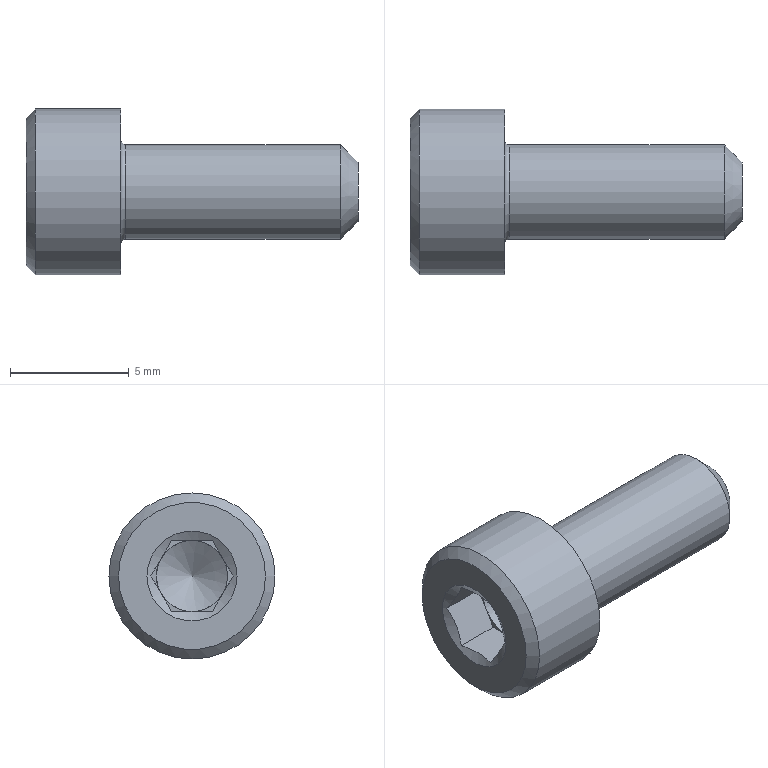Part | STEP file | Винт М4-6gx10 ГОСТ 11738-84 | 1 solid | 23 faces | box 14 x 7 x 7 mm | volume 252.721 mm3 | plane 15 | cone 4 | cylinder 3 | torus 1 | commonest cylinder face diameters 3 x1 4 x1 7 x1
STEP:
#1=CARTESIAN_POINT('',(-4.,3.1,0.));
#2=VERTEX_POINT('',#1);
#3=CARTESIAN_POINT('',(-4.,0.,0.));
#4=DIRECTION('',(1.,0.,0.));
#5=DIRECTION('',(0.,1.,0.));
#6=AXIS2_PLACEMENT_3D('',#3,#4,#5);
#7=CIRCLE('',#6,3.1);
#8=EDGE_CURVE('',#2,#2,#7,.T.);
#9=ORIENTED_EDGE('',*,*,#8,.F.);
#10=EDGE_LOOP('',(#9));
#11=FACE_BOUND('',#10,.T.);
#12=CARTESIAN_POINT('',(-4.,1.9,0.));
#13=VERTEX_POINT('',#12);
#14=CARTESIAN_POINT('',(-4.,0.,0.));
#15=DIRECTION('',(1.,0.,0.));
#16=DIRECTION('',(0.,1.,0.));
#17=AXIS2_PLACEMENT_3D('',#14,#15,#16);
#18=CIRCLE('',#17,1.9);
#19=EDGE_CURVE('',#13,#13,#18,.T.);
#20=ORIENTED_EDGE('',*,*,#19,.T.);
#21=EDGE_LOOP('',(#20));
#22=FACE_BOUND('',#21,.T.);
#23=CARTESIAN_POINT('',(-4.,0.,0.));
#24=DIRECTION('',(-1.,0.,0.));
#25=DIRECTION('',(0.,1.,0.));
#26=AXIS2_PLACEMENT_3D('',#23,#24,#25);
#27=PLANE('',#26);
#28=ADVANCED_FACE('',(#11,#22),#27,.T.);
#29=CARTESIAN_POINT('',(-3.903,0.866,-1.5));
#30=VERTEX_POINT('',#29);
#31=CARTESIAN_POINT('',(-3.903,-0.866,-1.5));
#32=VERTEX_POINT('',#31);
#33=CARTESIAN_POINT('',(-3.903,0.866,-1.5));
#34=CARTESIAN_POINT('',(-3.9,0.8561,-1.5));
#35=CARTESIAN_POINT('',(-3.89,0.8205,-1.5));
#36=CARTESIAN_POINT('',(-3.88,0.7841,-1.5));
#37=CARTESIAN_POINT('',(-3.862,0.7149,-1.5));
#38=CARTESIAN_POINT('',(-3.851,0.6675,-1.5));
#39=CARTESIAN_POINT('',(-3.83,0.5736,-1.5));
#40=CARTESIAN_POINT('',(-3.816,0.5059,-1.5));
#41=CARTESIAN_POINT('',(-3.8,0.4061,-1.5));
#42=CARTESIAN_POINT('',(-3.789,0.3305,-1.5));
#43=CARTESIAN_POINT('',(-3.781,0.2553,-1.5));
#44=CARTESIAN_POINT('',(-3.776,0.1888,-1.5));
#45=CARTESIAN_POINT('',(-3.773,0.1381,-1.5));
#46=CARTESIAN_POINT('',(-3.771,0.09396,-1.5));
#47=CARTESIAN_POINT('',(-3.77,0.0601,-1.5));
#48=CARTESIAN_POINT('',(-3.769,0.0279,-1.5));
#49=CARTESIAN_POINT('',(-3.769,-0.005342,-1.5));
#50=CARTESIAN_POINT('',(-3.769,-0.03809,-1.5));
#51=CARTESIAN_POINT('',(-3.77,-0.07339,-1.5));
#52=CARTESIAN_POINT('',(-3.771,-0.1059,-1.5));
#53=CARTESIAN_POINT('',(-3.773,-0.1382,-1.5));
#54=CARTESIAN_POINT('',(-3.775,-0.1786,-1.5));
#55=CARTESIAN_POINT('',(-3.779,-0.2268,-1.5));
#56=CARTESIAN_POINT('',(-3.783,-0.2747,-1.5));
#57=CARTESIAN_POINT('',(-3.788,-0.3143,-1.5));
#58=CARTESIAN_POINT('',(-3.792,-0.346,-1.5));
#59=CARTESIAN_POINT('',(-3.796,-0.3774,-1.5));
#60=CARTESIAN_POINT('',(-3.802,-0.4165,-1.5));
#61=CARTESIAN_POINT('',(-3.809,-0.463,-1.5));
#62=CARTESIAN_POINT('',(-3.817,-0.5065,-1.5));
#63=CARTESIAN_POINT('',(-3.823,-0.5371,-1.5));
#64=CARTESIAN_POINT('',(-3.829,-0.5675,-1.5));
#65=CARTESIAN_POINT('',(-3.836,-0.6003,-1.5));
#66=CARTESIAN_POINT('',(-3.846,-0.6453,-1.5));
#67=CARTESIAN_POINT('',(-3.856,-0.69,-1.5));
#68=CARTESIAN_POINT('',(-3.865,-0.7249,-1.5));
#69=CARTESIAN_POINT('',(-3.872,-0.7544,-1.5));
#70=CARTESIAN_POINT('',(-3.88,-0.7837,-1.5));
#71=CARTESIAN_POINT('',(-3.891,-0.8224,-1.5));
#72=CARTESIAN_POINT('',(-3.899,-0.8515,-1.5));
#73=CARTESIAN_POINT('',(-3.903,-0.866,-1.5));
#74=B_SPLINE_CURVE_WITH_KNOTS('',3,(#33,#34,#35,#36,#37,#38,#39,#40,#41,#42,#43,#44,#45,#46,#47,#48,#49,#50,#51,#52,#53,#54,#55,#56,#57,#58,#59,#60,#61,#62,#63,#64,#65,#66,#67,#68,#69,#70,#71,#72,#73),.UNSPECIFIED.,.F.,.F.,(4,1,1,1,1,1,1,1,1,1,1,1,1,1,1,1,1,1,1,1,1,1,1,1,1,1,1,1,1,1,1,1,1,1,1,1,1,1,4),(0.,0.01755,0.06316,0.06435,0.1397,0.1462,0.2284,0.2575,0.3188,0.3585,0.3865,0.4328,0.4451,0.4618,0.4905,0.5,0.5185,0.5464,0.5602,0.574,0.6016,0.6291,0.6565,0.6838,0.6972,0.7109,0.7379,0.7646,0.7912,0.8132,0.8177,0.8441,0.8703,0.8963,0.9224,0.9317,0.9483,0.9741,1.),.UNSPECIFIED.);
#75=EDGE_CURVE('',#30,#32,#74,.T.);
#76=ORIENTED_EDGE('',*,*,#75,.T.);
#77=CARTESIAN_POINT('',(-2.,-0.866,-1.5));
#78=VERTEX_POINT('',#77);
#79=CARTESIAN_POINT('',(-2.,-0.866,-1.5));
#80=DIRECTION('',(-1.,0.,0.));
#81=VECTOR('',#80,1.);
#82=LINE('',#79,#81);
#83=EDGE_CURVE('',#78,#32,#82,.T.);
#84=ORIENTED_EDGE('',*,*,#83,.F.);
#85=CARTESIAN_POINT('',(-2.,0.,-1.5));
#86=VERTEX_POINT('',#85);
#87=CARTESIAN_POINT('',(-2.,0.,-1.5));
#88=DIRECTION('',(0.,-1.,0.));
#89=VECTOR('',#88,1.);
#90=LINE('',#87,#89);
#91=EDGE_CURVE('',#86,#78,#90,.T.);
#92=ORIENTED_EDGE('',*,*,#91,.F.);
#93=CARTESIAN_POINT('',(-2.,0.866,-1.5));
#94=VERTEX_POINT('',#93);
#95=CARTESIAN_POINT('',(-2.,0.866,-1.5));
#96=DIRECTION('',(0.,-1.,0.));
#97=VECTOR('',#96,1.);
#98=LINE('',#95,#97);
#99=EDGE_CURVE('',#94,#86,#98,.T.);
#100=ORIENTED_EDGE('',*,*,#99,.F.);
#101=CARTESIAN_POINT('',(-2.,0.866,-1.5));
#102=DIRECTION('',(-1.,0.,0.));
#103=VECTOR('',#102,1.);
#104=LINE('',#101,#103);
#105=EDGE_CURVE('',#94,#30,#104,.T.);
#106=ORIENTED_EDGE('',*,*,#105,.T.);
#107=EDGE_LOOP('',(#76,#84,#92,#100,#106));
#108=FACE_BOUND('',#107,.T.);
#109=CARTESIAN_POINT('',(-2.,0.866,-1.5));
#110=DIRECTION('',(0.,0.,-1.));
#111=DIRECTION('',(0.,-1.,0.));
#112=AXIS2_PLACEMENT_3D('',#109,#110,#111);
#113=PLANE('',#112);
#114=ADVANCED_FACE('',(#108),#113,.F.);
#115=CARTESIAN_POINT('',(-3.903,-1.732,0.));
#116=VERTEX_POINT('',#115);
#117=CARTESIAN_POINT('',(-3.903,-0.866,-1.5));
#118=CARTESIAN_POINT('',(-3.893,-0.8838,-1.469));
#119=CARTESIAN_POINT('',(-3.871,-0.9233,-1.401));
#120=CARTESIAN_POINT('',(-3.839,-0.9883,-1.288));
#121=CARTESIAN_POINT('',(-3.81,-1.062,-1.161));
#122=CARTESIAN_POINT('',(-3.789,-1.133,-1.037));
#123=CARTESIAN_POINT('',(-3.777,-1.193,-0.9336));
#124=CARTESIAN_POINT('',(-3.772,-1.235,-0.8611));
#125=CARTESIAN_POINT('',(-3.77,-1.265,-0.8083));
#126=CARTESIAN_POINT('',(-3.769,-1.285,-0.7742));
#127=CARTESIAN_POINT('',(-3.769,-1.302,-0.7454));
#128=CARTESIAN_POINT('',(-3.769,-1.318,-0.717));
#129=CARTESIAN_POINT('',(-3.77,-1.34,-0.6794));
#130=CARTESIAN_POINT('',(-3.772,-1.364,-0.6373));
#131=CARTESIAN_POINT('',(-3.775,-1.388,-0.5954));
#132=CARTESIAN_POINT('',(-3.779,-1.412,-0.5536));
#133=CARTESIAN_POINT('',(-3.783,-1.436,-0.5121));
#134=CARTESIAN_POINT('',(-3.789,-1.46,-0.4709));
#135=CARTESIAN_POINT('',(-3.795,-1.484,-0.4299));
#136=CARTESIAN_POINT('',(-3.802,-1.507,-0.3893));
#137=CARTESIAN_POINT('',(-3.809,-1.531,-0.349));
#138=CARTESIAN_POINT('',(-3.817,-1.554,-0.3091));
#139=CARTESIAN_POINT('',(-3.826,-1.576,-0.2695));
#140=CARTESIAN_POINT('',(-3.836,-1.599,-0.2301));
#141=CARTESIAN_POINT('',(-3.846,-1.622,-0.1912));
#142=CARTESIAN_POINT('',(-3.856,-1.644,-0.1525));
#143=CARTESIAN_POINT('',(-3.867,-1.666,-0.114));
#144=CARTESIAN_POINT('',(-3.879,-1.688,-0.07582));
#145=CARTESIAN_POINT('',(-3.891,-1.71,-0.03781));
#146=CARTESIAN_POINT('',(-3.899,-1.725,-0.01258));
#147=CARTESIAN_POINT('',(-3.903,-1.732,0.));
#148=B_SPLINE_CURVE_WITH_KNOTS('',3,(#117,#118,#119,#120,#121,#122,#123,#124,#125,#126,#127,#128,#129,#130,#131,#132,#133,#134,#135,#136,#137,#138,#139,#140,#141,#142,#143,#144,#145,#146,#147),.UNSPECIFIED.,.F.,.F.,(4,1,1,1,1,1,1,1,1,1,1,1,1,1,1,1,1,1,1,1,1,1,1,1,1,1,1,1,4),(0.,0.06316,0.1397,0.2284,0.3188,0.3865,0.4328,0.4618,0.4905,0.5,0.5185,0.5464,0.574,0.6016,0.6291,0.6565,0.6838,0.7109,0.7379,0.7646,0.7912,0.8177,0.8441,0.8703,0.8963,0.9224,0.9483,0.9741,1.),.UNSPECIFIED.);
#149=EDGE_CURVE('',#32,#116,#148,.T.);
#150=ORIENTED_EDGE('',*,*,#149,.T.);
#151=CARTESIAN_POINT('',(-2.,-1.732,0.));
#152=VERTEX_POINT('',#151);
#153=CARTESIAN_POINT('',(-2.,-1.732,0.));
#154=DIRECTION('',(-1.,0.,0.));
#155=VECTOR('',#154,1.);
#156=LINE('',#153,#155);
#157=EDGE_CURVE('',#152,#116,#156,.T.);
#158=ORIENTED_EDGE('',*,*,#157,.F.);
#159=CARTESIAN_POINT('',(-2.,-1.299,-0.75));
#160=VERTEX_POINT('',#159);
#161=CARTESIAN_POINT('',(-2.,-1.299,-0.75));
#162=DIRECTION('',(0.,-0.5,0.866));
#163=VECTOR('',#162,1.);
#164=LINE('',#161,#163);
#165=EDGE_CURVE('',#160,#152,#164,.T.);
#166=ORIENTED_EDGE('',*,*,#165,.F.);
#167=CARTESIAN_POINT('',(-2.,-0.866,-1.5));
#168=DIRECTION('',(0.,-0.5,0.866));
#169=VECTOR('',#168,1.);
#170=LINE('',#167,#169);
#171=EDGE_CURVE('',#78,#160,#170,.T.);
#172=ORIENTED_EDGE('',*,*,#171,.F.);
#173=ORIENTED_EDGE('',*,*,#83,.T.);
#174=EDGE_LOOP('',(#150,#158,#166,#172,#173));
#175=FACE_BOUND('',#174,.T.);
#176=CARTESIAN_POINT('',(-2.,-0.866,-1.5));
#177=DIRECTION('',(0.,-0.866,-0.5));
#178=DIRECTION('',(0.,-0.5,0.866));
#179=AXIS2_PLACEMENT_3D('',#176,#177,#178);
#180=PLANE('',#179);
#181=ADVANCED_FACE('',(#175),#180,.F.);
#182=CARTESIAN_POINT('',(-3.903,-0.866,1.5));
#183=VERTEX_POINT('',#182);
#184=CARTESIAN_POINT('',(-3.903,-1.732,0.));
#185=CARTESIAN_POINT('',(-3.893,-1.714,0.0308));
#186=CARTESIAN_POINT('',(-3.871,-1.675,0.09916));
#187=CARTESIAN_POINT('',(-3.839,-1.61,0.2118));
#188=CARTESIAN_POINT('',(-3.81,-1.536,0.3391));
#189=CARTESIAN_POINT('',(-3.789,-1.465,0.4631));
#190=CARTESIAN_POINT('',(-3.777,-1.405,0.5664));
#191=CARTESIAN_POINT('',(-3.772,-1.363,0.6389));
#192=CARTESIAN_POINT('',(-3.77,-1.333,0.6917));
#193=CARTESIAN_POINT('',(-3.769,-1.313,0.7258));
#194=CARTESIAN_POINT('',(-3.769,-1.296,0.7546));
#195=CARTESIAN_POINT('',(-3.769,-1.28,0.783));
#196=CARTESIAN_POINT('',(-3.77,-1.258,0.8206));
#197=CARTESIAN_POINT('',(-3.772,-1.234,0.8627));
#198=CARTESIAN_POINT('',(-3.775,-1.21,0.9046));
#199=CARTESIAN_POINT('',(-3.779,-1.186,0.9464));
#200=CARTESIAN_POINT('',(-3.783,-1.162,0.9879));
#201=CARTESIAN_POINT('',(-3.789,-1.138,1.029));
#202=CARTESIAN_POINT('',(-3.795,-1.114,1.07));
#203=CARTESIAN_POINT('',(-3.802,-1.091,1.111));
#204=CARTESIAN_POINT('',(-3.809,-1.068,1.151));
#205=CARTESIAN_POINT('',(-3.817,-1.044,1.191));
#206=CARTESIAN_POINT('',(-3.826,-1.022,1.231));
#207=CARTESIAN_POINT('',(-3.836,-0.9989,1.27));
#208=CARTESIAN_POINT('',(-3.846,-0.9764,1.309));
#209=CARTESIAN_POINT('',(-3.856,-0.954,1.348));
#210=CARTESIAN_POINT('',(-3.867,-0.9319,1.386));
#211=CARTESIAN_POINT('',(-3.879,-0.9098,1.424));
#212=CARTESIAN_POINT('',(-3.891,-0.8879,1.462));
#213=CARTESIAN_POINT('',(-3.899,-0.8733,1.487));
#214=CARTESIAN_POINT('',(-3.903,-0.866,1.5));
#215=B_SPLINE_CURVE_WITH_KNOTS('',3,(#184,#185,#186,#187,#188,#189,#190,#191,#192,#193,#194,#195,#196,#197,#198,#199,#200,#201,#202,#203,#204,#205,#206,#207,#208,#209,#210,#211,#212,#213,#214),.UNSPECIFIED.,.F.,.F.,(4,1,1,1,1,1,1,1,1,1,1,1,1,1,1,1,1,1,1,1,1,1,1,1,1,1,1,1,4),(0.,0.06316,0.1397,0.2284,0.3188,0.3865,0.4328,0.4618,0.4905,0.5,0.5185,0.5464,0.574,0.6016,0.6291,0.6565,0.6838,0.7109,0.7379,0.7646,0.7912,0.8177,0.8441,0.8703,0.8963,0.9224,0.9483,0.9741,1.),.UNSPECIFIED.);
#216=EDGE_CURVE('',#116,#183,#215,.T.);
#217=ORIENTED_EDGE('',*,*,#216,.T.);
#218=CARTESIAN_POINT('',(-2.,-0.866,1.5));
#219=VERTEX_POINT('',#218);
#220=CARTESIAN_POINT('',(-2.,-0.866,1.5));
#221=DIRECTION('',(-1.,0.,0.));
#222=VECTOR('',#221,1.);
#223=LINE('',#220,#222);
#224=EDGE_CURVE('',#219,#183,#223,.T.);
#225=ORIENTED_EDGE('',*,*,#224,.F.);
#226=CARTESIAN_POINT('',(-2.,-1.299,0.75));
#227=VERTEX_POINT('',#226);
#228=CARTESIAN_POINT('',(-2.,-1.299,0.75));
#229=DIRECTION('',(0.,0.5,0.866));
#230=VECTOR('',#229,1.);
#231=LINE('',#228,#230);
#232=EDGE_CURVE('',#227,#219,#231,.T.);
#233=ORIENTED_EDGE('',*,*,#232,.F.);
#234=CARTESIAN_POINT('',(-2.,-1.732,0.));
#235=DIRECTION('',(0.,0.5,0.866));
#236=VECTOR('',#235,1.);
#237=LINE('',#234,#236);
#238=EDGE_CURVE('',#152,#227,#237,.T.);
#239=ORIENTED_EDGE('',*,*,#238,.F.);
#240=ORIENTED_EDGE('',*,*,#157,.T.);
#241=EDGE_LOOP('',(#217,#225,#233,#239,#240));
#242=FACE_BOUND('',#241,.T.);
#243=CARTESIAN_POINT('',(-2.,-1.732,0.));
#244=DIRECTION('',(0.,-0.866,0.5));
#245=DIRECTION('',(0.,0.5,0.866));
#246=AXIS2_PLACEMENT_3D('',#243,#244,#245);
#247=PLANE('',#246);
#248=ADVANCED_FACE('',(#242),#247,.F.);
#249=CARTESIAN_POINT('',(-3.903,0.866,1.5));
#250=VERTEX_POINT('',#249);
#251=CARTESIAN_POINT('',(-3.903,-0.866,1.5));
#252=CARTESIAN_POINT('',(-3.9,-0.8561,1.5));
#253=CARTESIAN_POINT('',(-3.89,-0.8205,1.5));
#254=CARTESIAN_POINT('',(-3.88,-0.7841,1.5));
#255=CARTESIAN_POINT('',(-3.862,-0.7149,1.5));
#256=CARTESIAN_POINT('',(-3.851,-0.6675,1.5));
#257=CARTESIAN_POINT('',(-3.83,-0.5736,1.5));
#258=CARTESIAN_POINT('',(-3.816,-0.5059,1.5));
#259=CARTESIAN_POINT('',(-3.8,-0.4061,1.5));
#260=CARTESIAN_POINT('',(-3.789,-0.3305,1.5));
#261=CARTESIAN_POINT('',(-3.781,-0.2553,1.5));
#262=CARTESIAN_POINT('',(-3.776,-0.1888,1.5));
#263=CARTESIAN_POINT('',(-3.773,-0.1381,1.5));
#264=CARTESIAN_POINT('',(-3.771,-0.09396,1.5));
#265=CARTESIAN_POINT('',(-3.77,-0.0601,1.5));
#266=CARTESIAN_POINT('',(-3.769,-0.0279,1.5));
#267=CARTESIAN_POINT('',(-3.769,0.005342,1.5));
#268=CARTESIAN_POINT('',(-3.769,0.03809,1.5));
#269=CARTESIAN_POINT('',(-3.77,0.07339,1.5));
#270=CARTESIAN_POINT('',(-3.771,0.1059,1.5));
#271=CARTESIAN_POINT('',(-3.773,0.1382,1.5));
#272=CARTESIAN_POINT('',(-3.775,0.1786,1.5));
#273=CARTESIAN_POINT('',(-3.779,0.2268,1.5));
#274=CARTESIAN_POINT('',(-3.783,0.2747,1.5));
#275=CARTESIAN_POINT('',(-3.788,0.3143,1.5));
#276=CARTESIAN_POINT('',(-3.792,0.346,1.5));
#277=CARTESIAN_POINT('',(-3.796,0.3774,1.5));
#278=CARTESIAN_POINT('',(-3.802,0.4165,1.5));
#279=CARTESIAN_POINT('',(-3.809,0.463,1.5));
#280=CARTESIAN_POINT('',(-3.817,0.5065,1.5));
#281=CARTESIAN_POINT('',(-3.823,0.5371,1.5));
#282=CARTESIAN_POINT('',(-3.829,0.5675,1.5));
#283=CARTESIAN_POINT('',(-3.836,0.6003,1.5));
#284=CARTESIAN_POINT('',(-3.846,0.6453,1.5));
#285=CARTESIAN_POINT('',(-3.856,0.69,1.5));
#286=CARTESIAN_POINT('',(-3.865,0.7249,1.5));
#287=CARTESIAN_POINT('',(-3.872,0.7544,1.5));
#288=CARTESIAN_POINT('',(-3.88,0.7837,1.5));
#289=CARTESIAN_POINT('',(-3.891,0.8224,1.5));
#290=CARTESIAN_POINT('',(-3.899,0.8515,1.5));
#291=CARTESIAN_POINT('',(-3.903,0.866,1.5));
#292=B_SPLINE_CURVE_WITH_KNOTS('',3,(#251,#252,#253,#254,#255,#256,#257,#258,#259,#260,#261,#262,#263,#264,#265,#266,#267,#268,#269,#270,#271,#272,#273,#274,#275,#276,#277,#278,#279,#280,#281,#282,#283,#284,#285,#286,#287,#288,#289,#290,#291),.UNSPECIFIED.,.F.,.F.,(4,1,1,1,1,1,1,1,1,1,1,1,1,1,1,1,1,1,1,1,1,1,1,1,1,1,1,1,1,1,1,1,1,1,1,1,1,1,4),(0.,0.01755,0.06316,0.06435,0.1397,0.1462,0.2284,0.2575,0.3188,0.3585,0.3865,0.4328,0.4451,0.4618,0.4905,0.5,0.5185,0.5464,0.5602,0.574,0.6016,0.6291,0.6565,0.6838,0.6972,0.7109,0.7379,0.7646,0.7912,0.8132,0.8177,0.8441,0.8703,0.8963,0.9224,0.9317,0.9483,0.9741,1.),.UNSPECIFIED.);
#293=EDGE_CURVE('',#183,#250,#292,.T.);
#294=ORIENTED_EDGE('',*,*,#293,.T.);
#295=CARTESIAN_POINT('',(-2.,0.866,1.5));
#296=VERTEX_POINT('',#295);
#297=CARTESIAN_POINT('',(-2.,0.866,1.5));
#298=DIRECTION('',(-1.,0.,0.));
#299=VECTOR('',#298,1.);
#300=LINE('',#297,#299);
#301=EDGE_CURVE('',#296,#250,#300,.T.);
#302=ORIENTED_EDGE('',*,*,#301,.F.);
#303=CARTESIAN_POINT('',(-2.,0.,1.5));
#304=VERTEX_POINT('',#303);
#305=CARTESIAN_POINT('',(-2.,0.,1.5));
#306=DIRECTION('',(0.,1.,0.));
#307=VECTOR('',#306,1.);
#308=LINE('',#305,#307);
#309=EDGE_CURVE('',#304,#296,#308,.T.);
#310=ORIENTED_EDGE('',*,*,#309,.F.);
#311=CARTESIAN_POINT('',(-2.,-0.866,1.5));
#312=DIRECTION('',(0.,1.,0.));
#313=VECTOR('',#312,1.);
#314=LINE('',#311,#313);
#315=EDGE_CURVE('',#219,#304,#314,.T.);
#316=ORIENTED_EDGE('',*,*,#315,.F.);
#317=ORIENTED_EDGE('',*,*,#224,.T.);
#318=EDGE_LOOP('',(#294,#302,#310,#316,#317));
#319=FACE_BOUND('',#318,.T.);
#320=CARTESIAN_POINT('',(-2.,-0.866,1.5));
#321=DIRECTION('',(0.,0.,1.));
#322=DIRECTION('',(0.,1.,0.));
#323=AXIS2_PLACEMENT_3D('',#320,#321,#322);
#324=PLANE('',#323);
#325=ADVANCED_FACE('',(#319),#324,.F.);
#326=CARTESIAN_POINT('',(-3.903,1.732,0.000000001));
#327=VERTEX_POINT('',#326);
#328=CARTESIAN_POINT('',(-3.903,1.732,0.));
#329=CARTESIAN_POINT('',(-3.893,1.714,-0.0308));
#330=CARTESIAN_POINT('',(-3.871,1.675,-0.09916));
#331=CARTESIAN_POINT('',(-3.839,1.61,-0.2118));
#332=CARTESIAN_POINT('',(-3.81,1.536,-0.3391));
#333=CARTESIAN_POINT('',(-3.789,1.465,-0.4631));
#334=CARTESIAN_POINT('',(-3.777,1.405,-0.5664));
#335=CARTESIAN_POINT('',(-3.772,1.363,-0.6389));
#336=CARTESIAN_POINT('',(-3.77,1.333,-0.6917));
#337=CARTESIAN_POINT('',(-3.769,1.313,-0.7258));
#338=CARTESIAN_POINT('',(-3.769,1.296,-0.7546));
#339=CARTESIAN_POINT('',(-3.769,1.28,-0.783));
#340=CARTESIAN_POINT('',(-3.77,1.258,-0.8206));
#341=CARTESIAN_POINT('',(-3.772,1.234,-0.8627));
#342=CARTESIAN_POINT('',(-3.775,1.21,-0.9046));
#343=CARTESIAN_POINT('',(-3.779,1.186,-0.9464));
#344=CARTESIAN_POINT('',(-3.783,1.162,-0.9879));
#345=CARTESIAN_POINT('',(-3.789,1.138,-1.029));
#346=CARTESIAN_POINT('',(-3.795,1.114,-1.07));
#347=CARTESIAN_POINT('',(-3.802,1.091,-1.111));
#348=CARTESIAN_POINT('',(-3.809,1.068,-1.151));
#349=CARTESIAN_POINT('',(-3.817,1.044,-1.191));
#350=CARTESIAN_POINT('',(-3.826,1.022,-1.231));
#351=CARTESIAN_POINT('',(-3.836,0.9989,-1.27));
#352=CARTESIAN_POINT('',(-3.846,0.9764,-1.309));
#353=CARTESIAN_POINT('',(-3.856,0.954,-1.348));
#354=CARTESIAN_POINT('',(-3.867,0.9319,-1.386));
#355=CARTESIAN_POINT('',(-3.879,0.9098,-1.424));
#356=CARTESIAN_POINT('',(-3.891,0.8879,-1.462));
#357=CARTESIAN_POINT('',(-3.899,0.8733,-1.487));
#358=CARTESIAN_POINT('',(-3.903,0.866,-1.5));
#359=B_SPLINE_CURVE_WITH_KNOTS('',3,(#328,#329,#330,#331,#332,#333,#334,#335,#336,#337,#338,#339,#340,#341,#342,#343,#344,#345,#346,#347,#348,#349,#350,#351,#352,#353,#354,#355,#356,#357,#358),.UNSPECIFIED.,.F.,.F.,(4,1,1,1,1,1,1,1,1,1,1,1,1,1,1,1,1,1,1,1,1,1,1,1,1,1,1,1,4),(0.,0.06315,0.1397,0.2284,0.3188,0.3865,0.4327,0.4618,0.4905,0.5,0.5185,0.5464,0.574,0.6016,0.6291,0.6565,0.6838,0.7109,0.7379,0.7646,0.7912,0.8177,0.8441,0.8703,0.8963,0.9224,0.9483,0.9741,1.),.UNSPECIFIED.);
#360=EDGE_CURVE('',#327,#30,#359,.T.);
#361=ORIENTED_EDGE('',*,*,#360,.T.);
#362=ORIENTED_EDGE('',*,*,#105,.F.);
#363=CARTESIAN_POINT('',(-2.,1.299,-0.75));
#364=VERTEX_POINT('',#363);
#365=CARTESIAN_POINT('',(-2.,1.299,-0.75));
#366=DIRECTION('',(0.,-0.5,-0.866));
#367=VECTOR('',#366,1.);
#368=LINE('',#365,#367);
#369=EDGE_CURVE('',#364,#94,#368,.T.);
#370=ORIENTED_EDGE('',*,*,#369,.F.);
#371=CARTESIAN_POINT('',(-2.,1.732,0.));
#372=VERTEX_POINT('',#371);
#373=CARTESIAN_POINT('',(-2.,1.732,0.));
#374=DIRECTION('',(0.,-0.5,-0.866));
#375=VECTOR('',#374,1.);
#376=LINE('',#373,#375);
#377=EDGE_CURVE('',#372,#364,#376,.T.);
#378=ORIENTED_EDGE('',*,*,#377,.F.);
#379=CARTESIAN_POINT('',(-2.,1.732,0.));
#380=DIRECTION('',(-1.,0.,0.));
#381=VECTOR('',#380,1.);
#382=LINE('',#379,#381);
#383=EDGE_CURVE('',#372,#327,#382,.T.);
#384=ORIENTED_EDGE('',*,*,#383,.T.);
#385=EDGE_LOOP('',(#361,#362,#370,#378,#384));
#386=FACE_BOUND('',#385,.T.);
#387=CARTESIAN_POINT('',(-2.,1.732,0.));
#388=DIRECTION('',(0.,0.866,-0.5));
#389=DIRECTION('',(0.,-0.5,-0.866));
#390=AXIS2_PLACEMENT_3D('',#387,#388,#389);
#391=PLANE('',#390);
#392=ADVANCED_FACE('',(#386),#391,.F.);
#393=CARTESIAN_POINT('',(-3.903,0.866,1.5));
#394=CARTESIAN_POINT('',(-3.893,0.8838,1.469));
#395=CARTESIAN_POINT('',(-3.871,0.9233,1.401));
#396=CARTESIAN_POINT('',(-3.839,0.9883,1.288));
#397=CARTESIAN_POINT('',(-3.81,1.062,1.161));
#398=CARTESIAN_POINT('',(-3.789,1.133,1.037));
#399=CARTESIAN_POINT('',(-3.777,1.193,0.9336));
#400=CARTESIAN_POINT('',(-3.772,1.235,0.8611));
#401=CARTESIAN_POINT('',(-3.77,1.265,0.8083));
#402=CARTESIAN_POINT('',(-3.769,1.285,0.7742));
#403=CARTESIAN_POINT('',(-3.769,1.302,0.7454));
#404=CARTESIAN_POINT('',(-3.769,1.318,0.717));
#405=CARTESIAN_POINT('',(-3.77,1.34,0.6794));
#406=CARTESIAN_POINT('',(-3.772,1.364,0.6373));
#407=CARTESIAN_POINT('',(-3.775,1.388,0.5954));
#408=CARTESIAN_POINT('',(-3.779,1.412,0.5536));
#409=CARTESIAN_POINT('',(-3.783,1.436,0.5121));
#410=CARTESIAN_POINT('',(-3.789,1.46,0.4709));
#411=CARTESIAN_POINT('',(-3.795,1.484,0.4299));
#412=CARTESIAN_POINT('',(-3.802,1.507,0.3893));
#413=CARTESIAN_POINT('',(-3.809,1.531,0.349));
#414=CARTESIAN_POINT('',(-3.817,1.554,0.3091));
#415=CARTESIAN_POINT('',(-3.826,1.576,0.2695));
#416=CARTESIAN_POINT('',(-3.836,1.599,0.2301));
#417=CARTESIAN_POINT('',(-3.846,1.622,0.1912));
#418=CARTESIAN_POINT('',(-3.856,1.644,0.1525));
#419=CARTESIAN_POINT('',(-3.867,1.666,0.114));
#420=CARTESIAN_POINT('',(-3.879,1.688,0.07582));
#421=CARTESIAN_POINT('',(-3.891,1.71,0.03781));
#422=CARTESIAN_POINT('',(-3.899,1.725,0.01258));
#423=CARTESIAN_POINT('',(-3.903,1.732,0.000000005));
#424=B_SPLINE_CURVE_WITH_KNOTS('',3,(#393,#394,#395,#396,#397,#398,#399,#400,#401,#402,#403,#404,#405,#406,#407,#408,#409,#410,#411,#412,#413,#414,#415,#416,#417,#418,#419,#420,#421,#422,#423),.UNSPECIFIED.,.F.,.F.,(4,1,1,1,1,1,1,1,1,1,1,1,1,1,1,1,1,1,1,1,1,1,1,1,1,1,1,1,4),(0.,0.06315,0.1397,0.2284,0.3188,0.3865,0.4327,0.4618,0.4905,0.5,0.5185,0.5464,0.574,0.6016,0.6291,0.6565,0.6838,0.7109,0.7379,0.7646,0.7912,0.8177,0.8441,0.8703,0.8963,0.9224,0.9483,0.9741,1.),.UNSPECIFIED.);
#425=EDGE_CURVE('',#250,#327,#424,.T.);
#426=ORIENTED_EDGE('',*,*,#425,.T.);
#427=ORIENTED_EDGE('',*,*,#383,.F.);
#428=CARTESIAN_POINT('',(-2.,1.299,0.75));
#429=VERTEX_POINT('',#428);
#430=CARTESIAN_POINT('',(-2.,1.299,0.75));
#431=DIRECTION('',(0.,0.5,-0.866));
#432=VECTOR('',#431,1.);
#433=LINE('',#430,#432);
#434=EDGE_CURVE('',#429,#372,#433,.T.);
#435=ORIENTED_EDGE('',*,*,#434,.F.);
#436=CARTESIAN_POINT('',(-2.,0.866,1.5));
#437=DIRECTION('',(0.,0.5,-0.866));
#438=VECTOR('',#437,1.);
#439=LINE('',#436,#438);
#440=EDGE_CURVE('',#296,#429,#439,.T.);
#441=ORIENTED_EDGE('',*,*,#440,.F.);
#442=ORIENTED_EDGE('',*,*,#301,.T.);
#443=EDGE_LOOP('',(#426,#427,#435,#441,#442));
#444=FACE_BOUND('',#443,.T.);
#445=CARTESIAN_POINT('',(-2.,0.866,1.5));
#446=DIRECTION('',(0.,0.866,0.5));
#447=DIRECTION('',(0.,0.5,-0.866));
#448=AXIS2_PLACEMENT_3D('',#445,#446,#447);
#449=PLANE('',#448);
#450=ADVANCED_FACE('',(#444),#449,.F.);
#451=ORIENTED_EDGE('',*,*,#425,.F.);
#452=ORIENTED_EDGE('',*,*,#293,.F.);
#453=ORIENTED_EDGE('',*,*,#216,.F.);
#454=ORIENTED_EDGE('',*,*,#149,.F.);
#455=ORIENTED_EDGE('',*,*,#75,.F.);
#456=ORIENTED_EDGE('',*,*,#360,.F.);
#457=EDGE_LOOP('',(#451,#452,#453,#454,#455,#456));
#458=FACE_BOUND('',#457,.T.);
#459=ORIENTED_EDGE('',*,*,#19,.F.);
#460=EDGE_LOOP('',(#459));
#461=FACE_OUTER_BOUND('',#460,.T.);
#462=CARTESIAN_POINT('',(-3.885,0.,0.));
#463=DIRECTION('',(-1.,0.,0.));
#464=DIRECTION('',(0.,-1.,0.));
#465=AXIS2_PLACEMENT_3D('',#462,#463,#464);
#466=CONICAL_SURFACE('',#465,1.7,1.047);
#467=ADVANCED_FACE('',(#458,#461),#466,.F.);
#468=CARTESIAN_POINT('',(-3.6,3.5,0.));
#469=VERTEX_POINT('',#468);
#470=CARTESIAN_POINT('',(-3.6,0.,0.));
#471=DIRECTION('',(1.,0.,0.));
#472=DIRECTION('',(0.,1.,0.));
#473=AXIS2_PLACEMENT_3D('',#470,#471,#472);
#474=CIRCLE('',#473,3.5);
#475=EDGE_CURVE('',#469,#469,#474,.T.);
#476=ORIENTED_EDGE('',*,*,#475,.F.);
#477=EDGE_LOOP('',(#476));
#478=FACE_OUTER_BOUND('',#477,.T.);
#479=ORIENTED_EDGE('',*,*,#8,.T.);
#480=EDGE_LOOP('',(#479));
#481=FACE_OUTER_BOUND('',#480,.T.);
#482=CARTESIAN_POINT('',(-3.8,0.,0.));
#483=DIRECTION('',(1.,0.,0.));
#484=DIRECTION('',(0.,1.,0.));
#485=AXIS2_PLACEMENT_3D('',#482,#483,#484);
#486=CONICAL_SURFACE('',#485,3.3,0.7854);
#487=ADVANCED_FACE('',(#478,#481),#486,.T.);
#488=CARTESIAN_POINT('',(-2.,0.,0.));
#489=DIRECTION('',(1.,0.,0.));
#490=DIRECTION('',(0.,-0.866,-0.5));
#491=AXIS2_PLACEMENT_3D('',#488,#489,#490);
#492=CIRCLE('',#491,1.5);
#493=EDGE_CURVE('',#160,#86,#492,.T.);
#494=ORIENTED_EDGE('',*,*,#493,.T.);
#495=ORIENTED_EDGE('',*,*,#91,.T.);
#496=ORIENTED_EDGE('',*,*,#171,.T.);
#497=EDGE_LOOP('',(#494,#495,#496));
#498=FACE_BOUND('',#497,.T.);
#499=CARTESIAN_POINT('',(-2.,0.,0.));
#500=DIRECTION('',(-1.,0.,0.));
#501=DIRECTION('',(0.,0.,-1.));
#502=AXIS2_PLACEMENT_3D('',#499,#500,#501);
#503=PLANE('',#502);
#504=ADVANCED_FACE('',(#498),#503,.T.);
#505=CARTESIAN_POINT('',(-2.,0.,0.));
#506=DIRECTION('',(1.,0.,0.));
#507=DIRECTION('',(0.,0.,-1.));
#508=AXIS2_PLACEMENT_3D('',#505,#506,#507);
#509=CIRCLE('',#508,1.5);
#510=EDGE_CURVE('',#86,#364,#509,.T.);
#511=ORIENTED_EDGE('',*,*,#510,.T.);
#512=ORIENTED_EDGE('',*,*,#369,.T.);
#513=ORIENTED_EDGE('',*,*,#99,.T.);
#514=EDGE_LOOP('',(#511,#512,#513));
#515=FACE_BOUND('',#514,.T.);
#516=CARTESIAN_POINT('',(-2.,0.,0.));
#517=DIRECTION('',(-1.,0.,0.));
#518=DIRECTION('',(0.,0.,-1.));
#519=AXIS2_PLACEMENT_3D('',#516,#517,#518);
#520=PLANE('',#519);
#521=ADVANCED_FACE('',(#515),#520,.T.);
#522=CARTESIAN_POINT('',(-2.,0.,0.));
#523=DIRECTION('',(1.,0.,0.));
#524=DIRECTION('',(0.,-0.866,0.5));
#525=AXIS2_PLACEMENT_3D('',#522,#523,#524);
#526=CIRCLE('',#525,1.5);
#527=EDGE_CURVE('',#227,#160,#526,.T.);
#528=ORIENTED_EDGE('',*,*,#527,.T.);
#529=ORIENTED_EDGE('',*,*,#165,.T.);
#530=ORIENTED_EDGE('',*,*,#238,.T.);
#531=EDGE_LOOP('',(#528,#529,#530));
#532=FACE_BOUND('',#531,.T.);
#533=CARTESIAN_POINT('',(-2.,0.,0.));
#534=DIRECTION('',(-1.,0.,0.));
#535=DIRECTION('',(0.,0.,-1.));
#536=AXIS2_PLACEMENT_3D('',#533,#534,#535);
#537=PLANE('',#536);
#538=ADVANCED_FACE('',(#532),#537,.T.);
#539=CARTESIAN_POINT('',(-2.,0.,0.));
#540=DIRECTION('',(1.,0.,0.));
#541=DIRECTION('',(0.,0.,1.));
#542=AXIS2_PLACEMENT_3D('',#539,#540,#541);
#543=CIRCLE('',#542,1.5);
#544=EDGE_CURVE('',#304,#227,#543,.T.);
#545=ORIENTED_EDGE('',*,*,#544,.T.);
#546=ORIENTED_EDGE('',*,*,#232,.T.);
#547=ORIENTED_EDGE('',*,*,#315,.T.);
#548=EDGE_LOOP('',(#545,#546,#547));
#549=FACE_BOUND('',#548,.T.);
#550=CARTESIAN_POINT('',(-2.,0.,0.));
#551=DIRECTION('',(-1.,0.,0.));
#552=DIRECTION('',(0.,0.,-1.));
#553=AXIS2_PLACEMENT_3D('',#550,#551,#552);
#554=PLANE('',#553);
#555=ADVANCED_FACE('',(#549),#554,.T.);
#556=CARTESIAN_POINT('',(-2.,0.,0.));
#557=DIRECTION('',(1.,0.,0.));
#558=DIRECTION('',(0.,0.866,0.5));
#559=AXIS2_PLACEMENT_3D('',#556,#557,#558);
#560=CIRCLE('',#559,1.5);
#561=EDGE_CURVE('',#429,#304,#560,.T.);
#562=ORIENTED_EDGE('',*,*,#561,.T.);
#563=ORIENTED_EDGE('',*,*,#309,.T.);
#564=ORIENTED_EDGE('',*,*,#440,.T.);
#565=EDGE_LOOP('',(#562,#563,#564));
#566=FACE_BOUND('',#565,.T.);
#567=CARTESIAN_POINT('',(-2.,0.,0.));
#568=DIRECTION('',(-1.,0.,0.));
#569=DIRECTION('',(0.,0.,-1.));
#570=AXIS2_PLACEMENT_3D('',#567,#568,#569);
#571=PLANE('',#570);
#572=ADVANCED_FACE('',(#566),#571,.T.);
#573=CARTESIAN_POINT('',(-2.,1.5,0.));
#574=VERTEX_POINT('',#573);
#575=CARTESIAN_POINT('',(-2.,0.,0.));
#576=DIRECTION('',(1.,0.,0.));
#577=DIRECTION('',(0.,1.,0.));
#578=AXIS2_PLACEMENT_3D('',#575,#576,#577);
#579=CIRCLE('',#578,1.5);
#580=EDGE_CURVE('',#574,#429,#579,.T.);
#581=ORIENTED_EDGE('',*,*,#580,.T.);
#582=ORIENTED_EDGE('',*,*,#434,.T.);
#583=ORIENTED_EDGE('',*,*,#377,.T.);
#584=CARTESIAN_POINT('',(-2.,0.,0.));
#585=DIRECTION('',(1.,0.,0.));
#586=DIRECTION('',(0.,0.866,-0.5));
#587=AXIS2_PLACEMENT_3D('',#584,#585,#586);
#588=CIRCLE('',#587,1.5);
#589=EDGE_CURVE('',#364,#574,#588,.T.);
#590=ORIENTED_EDGE('',*,*,#589,.T.);
#591=EDGE_LOOP('',(#581,#582,#583,#590));
#592=FACE_BOUND('',#591,.T.);
#593=CARTESIAN_POINT('',(-2.,0.,0.));
#594=DIRECTION('',(-1.,0.,0.));
#595=DIRECTION('',(0.,0.,-1.));
#596=AXIS2_PLACEMENT_3D('',#593,#594,#595);
#597=PLANE('',#596);
#598=ADVANCED_FACE('',(#592),#597,.T.);
#599=CARTESIAN_POINT('',(0.,3.5,0.));
#600=VERTEX_POINT('',#599);
#601=CARTESIAN_POINT('',(0.,0.,0.));
#602=DIRECTION('',(1.,0.,0.));
#603=DIRECTION('',(0.,1.,0.));
#604=AXIS2_PLACEMENT_3D('',#601,#602,#603);
#605=CIRCLE('',#604,3.5);
#606=EDGE_CURVE('',#600,#600,#605,.T.);
#607=ORIENTED_EDGE('',*,*,#606,.F.);
#608=EDGE_LOOP('',(#607));
#609=FACE_OUTER_BOUND('',#608,.T.);
#610=ORIENTED_EDGE('',*,*,#475,.T.);
#611=EDGE_LOOP('',(#610));
#612=FACE_OUTER_BOUND('',#611,.T.);
#613=CARTESIAN_POINT('',(-4.,0.,0.));
#614=DIRECTION('',(1.,0.,0.));
#615=DIRECTION('',(0.,1.,0.));
#616=AXIS2_PLACEMENT_3D('',#613,#614,#615);
#617=CYLINDRICAL_SURFACE('',#616,3.5);
#618=ADVANCED_FACE('',(#609,#612),#617,.T.);
#619=CARTESIAN_POINT('',(-1.4,1.5,0.));
#620=VERTEX_POINT('',#619);
#621=CARTESIAN_POINT('',(-1.4,0.,0.));
#622=DIRECTION('',(1.,0.,0.));
#623=DIRECTION('',(0.,1.,0.));
#624=AXIS2_PLACEMENT_3D('',#621,#622,#623);
#625=CIRCLE('',#624,1.5);
#626=EDGE_CURVE('',#620,#620,#625,.T.);
#627=ORIENTED_EDGE('',*,*,#626,.T.);
#628=EDGE_LOOP('',(#627));
#629=FACE_OUTER_BOUND('',#628,.T.);
#630=ORIENTED_EDGE('',*,*,#589,.F.);
#631=ORIENTED_EDGE('',*,*,#510,.F.);
#632=ORIENTED_EDGE('',*,*,#493,.F.);
#633=ORIENTED_EDGE('',*,*,#527,.F.);
#634=ORIENTED_EDGE('',*,*,#544,.F.);
#635=ORIENTED_EDGE('',*,*,#561,.F.);
#636=ORIENTED_EDGE('',*,*,#580,.F.);
#637=EDGE_LOOP('',(#630,#631,#632,#633,#634,#635,#636));
#638=FACE_BOUND('',#637,.T.);
#639=CARTESIAN_POINT('',(-4.,0.,0.));
#640=DIRECTION('',(1.,0.,0.));
#641=DIRECTION('',(0.,1.,0.));
#642=AXIS2_PLACEMENT_3D('',#639,#640,#641);
#643=CYLINDRICAL_SURFACE('',#642,1.5);
#644=ADVANCED_FACE('',(#629,#638),#643,.F.);
#645=ORIENTED_EDGE('',*,*,#606,.T.);
#646=EDGE_LOOP('',(#645));
#647=FACE_BOUND('',#646,.T.);
#648=CARTESIAN_POINT('',(0.,0.,-2.2));
#649=VERTEX_POINT('',#648);
#650=CARTESIAN_POINT('',(0.,0.,0.));
#651=DIRECTION('',(-1.,0.,0.));
#652=DIRECTION('',(0.,0.,-1.));
#653=AXIS2_PLACEMENT_3D('',#650,#651,#652);
#654=CIRCLE('',#653,2.2);
#655=EDGE_CURVE('',#649,#649,#654,.T.);
#656=ORIENTED_EDGE('',*,*,#655,.T.);
#657=EDGE_LOOP('',(#656));
#658=FACE_BOUND('',#657,.T.);
#659=CARTESIAN_POINT('',(0.,0.,0.));
#660=DIRECTION('',(1.,0.,0.));
#661=DIRECTION('',(0.,1.,0.));
#662=AXIS2_PLACEMENT_3D('',#659,#660,#661);
#663=PLANE('',#662);
#664=ADVANCED_FACE('',(#647,#658),#663,.T.);
#665=ORIENTED_EDGE('',*,*,#626,.F.);
#666=EDGE_LOOP('',(#665));
#667=FACE_OUTER_BOUND('',#666,.T.);
#668=CARTESIAN_POINT('',(-0.967,0.,0.));
#669=DIRECTION('',(-1.,0.,0.));
#670=DIRECTION('',(0.,-1.,0.));
#671=AXIS2_PLACEMENT_3D('',#668,#669,#670);
#672=CONICAL_SURFACE('',#671,0.75,1.047);
#673=ADVANCED_FACE('',(#667),#672,.F.);
#674=CARTESIAN_POINT('',(0.2,0.,-2.));
#675=VERTEX_POINT('',#674);
#676=CARTESIAN_POINT('',(0.2,0.,0.));
#677=DIRECTION('',(-1.,0.,0.));
#678=DIRECTION('',(0.,0.,-1.));
#679=AXIS2_PLACEMENT_3D('',#676,#677,#678);
#680=CIRCLE('',#679,2.);
#681=EDGE_CURVE('',#675,#675,#680,.T.);
#682=ORIENTED_EDGE('',*,*,#681,.T.);
#683=EDGE_LOOP('',(#682));
#684=FACE_OUTER_BOUND('',#683,.T.);
#685=ORIENTED_EDGE('',*,*,#655,.F.);
#686=EDGE_LOOP('',(#685));
#687=FACE_OUTER_BOUND('',#686,.T.);
#688=CARTESIAN_POINT('',(0.2,0.,0.));
#689=DIRECTION('',(-1.,0.,0.));
#690=DIRECTION('',(0.,0.,-1.));
#691=AXIS2_PLACEMENT_3D('',#688,#689,#690);
#692=TOROIDAL_SURFACE('',#691,2.2,0.2);
#693=ADVANCED_FACE('',(#684,#687),#692,.F.);
#694=CARTESIAN_POINT('',(9.25,0.,-2.));
#695=VERTEX_POINT('',#694);
#696=CARTESIAN_POINT('',(9.25,0.,0.));
#697=DIRECTION('',(-1.,0.,0.));
#698=DIRECTION('',(0.,0.,-1.));
#699=AXIS2_PLACEMENT_3D('',#696,#697,#698);
#700=CIRCLE('',#699,2.);
#701=EDGE_CURVE('',#695,#695,#700,.T.);
#702=ORIENTED_EDGE('',*,*,#701,.T.);
#703=EDGE_LOOP('',(#702));
#704=FACE_OUTER_BOUND('',#703,.T.);
#705=ORIENTED_EDGE('',*,*,#681,.F.);
#706=EDGE_LOOP('',(#705));
#707=FACE_OUTER_BOUND('',#706,.T.);
#708=CARTESIAN_POINT('',(10.,0.,0.));
#709=DIRECTION('',(-1.,0.,0.));
#710=DIRECTION('',(0.,0.,-1.));
#711=AXIS2_PLACEMENT_3D('',#708,#709,#710);
#712=CYLINDRICAL_SURFACE('',#711,2.);
#713=ADVANCED_FACE('',(#704,#707),#712,.T.);
#714=CARTESIAN_POINT('',(10.,0.,-1.25));
#715=VERTEX_POINT('',#714);
#716=CARTESIAN_POINT('',(10.,0.,0.));
#717=DIRECTION('',(-1.,0.,0.));
#718=DIRECTION('',(0.,0.,-1.));
#719=AXIS2_PLACEMENT_3D('',#716,#717,#718);
#720=CIRCLE('',#719,1.25);
#721=EDGE_CURVE('',#715,#715,#720,.T.);
#722=ORIENTED_EDGE('',*,*,#721,.F.);
#723=EDGE_LOOP('',(#722));
#724=FACE_BOUND('',#723,.T.);
#725=CARTESIAN_POINT('',(10.,0.,0.));
#726=DIRECTION('',(-1.,0.,0.));
#727=DIRECTION('',(0.,0.,-1.));
#728=AXIS2_PLACEMENT_3D('',#725,#726,#727);
#729=PLANE('',#728);
#730=ADVANCED_FACE('',(#724),#729,.F.);
#731=ORIENTED_EDGE('',*,*,#721,.T.);
#732=EDGE_LOOP('',(#731));
#733=FACE_OUTER_BOUND('',#732,.T.);
#734=ORIENTED_EDGE('',*,*,#701,.F.);
#735=EDGE_LOOP('',(#734));
#736=FACE_OUTER_BOUND('',#735,.T.);
#737=CARTESIAN_POINT('',(9.625,0.,0.));
#738=DIRECTION('',(-1.,0.,0.));
#739=DIRECTION('',(0.,0.,-1.));
#740=AXIS2_PLACEMENT_3D('',#737,#738,#739);
#741=CONICAL_SURFACE('',#740,1.625,0.7854);
#742=ADVANCED_FACE('',(#733,#736),#741,.T.);
#743=CLOSED_SHELL('',(#28,#114,#181,#248,#325,#392,#450,#467,#487,#504,#521,#538,#555,#572,#598,#618,#644,#664,#673,#693,#713,#730,#742));
#744=MANIFOLD_SOLID_BREP('',#743);
#745=(LENGTH_UNIT()NAMED_UNIT(*)SI_UNIT(.MILLI.,.METRE.));
#746=UNCERTAINTY_MEASURE_WITH_UNIT(LENGTH_MEASURE(0.00001),#745,'','');
#747=(NAMED_UNIT(*)PLANE_ANGLE_UNIT()SI_UNIT($,.RADIAN.));
#748=(NAMED_UNIT(*)SI_UNIT($,.STERADIAN.)SOLID_ANGLE_UNIT());
#749=(GEOMETRIC_REPRESENTATION_CONTEXT(3)GLOBAL_UNCERTAINTY_ASSIGNED_CONTEXT((#746))GLOBAL_UNIT_ASSIGNED_CONTEXT((#745,#747,#748))REPRESENTATION_CONTEXT('',''));
#750=ADVANCED_BREP_SHAPE_REPRESENTATION('',(#744),#749);